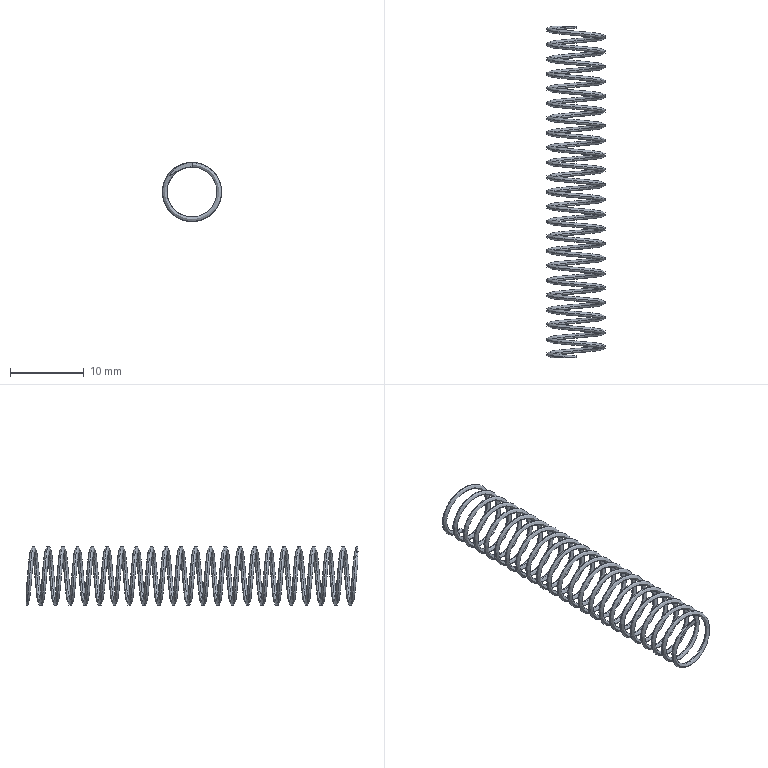Part | SolidWorks | features Helix 1, ICE 1, Sweep 1 | 1 solid | 6 faces | box 8 x 45 x 8 mm | volume 146.9 mm3 | plane 4 | spline 2